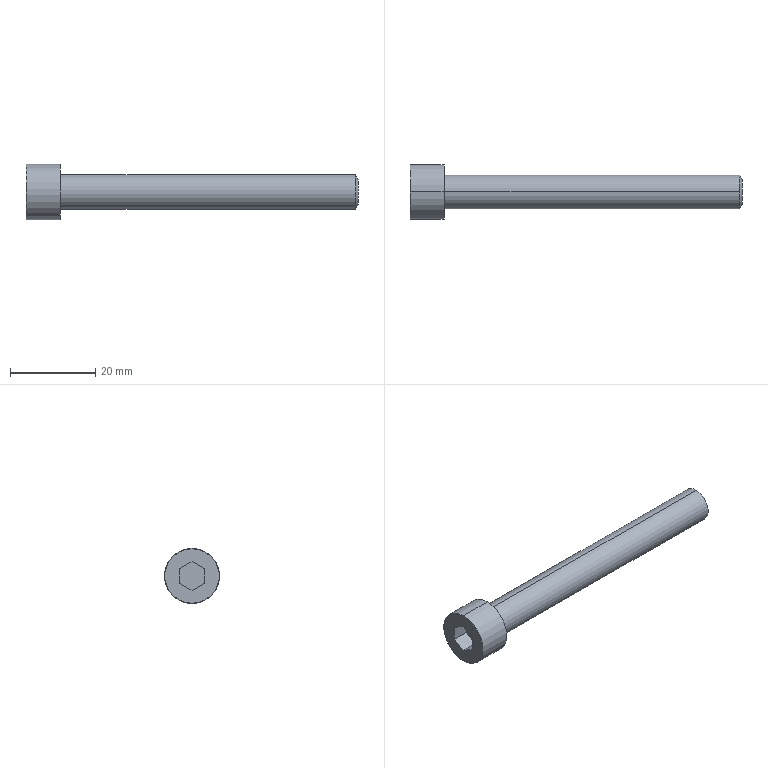Part | STEP file | 1 solid | 20 faces | box 78 x 13 x 13 mm | volume 4451 mm3 | plane 10 | torus 4 | cylinder 4 | cone 2 | commonest cylinder face diameters 8 x2 13 x2
STEP:
#1=CARTESIAN_POINT('',(0.,0.,6.4));
#2=VERTEX_POINT('',#1);
#3=CARTESIAN_POINT('',(0.,0.,-6.4));
#4=VERTEX_POINT('',#3);
#5=CARTESIAN_POINT('',(0.,0.,0.));
#6=DIRECTION('',(-1.,0.,0.));
#7=DIRECTION('',(0.,0.,-1.));
#8=AXIS2_PLACEMENT_3D('',#5,#6,#7);
#9=CIRCLE('',#8,6.4);
#10=EDGE_CURVE('',#2,#4,#9,.T.);
#11=ORIENTED_EDGE('',*,*,#10,.F.);
#12=CARTESIAN_POINT('',(0.1,0.,6.5));
#13=VERTEX_POINT('',#12);
#14=CARTESIAN_POINT('',(0.1,0.,6.4));
#15=DIRECTION('',(0.,1.,0.));
#16=DIRECTION('',(0.,0.,1.));
#17=AXIS2_PLACEMENT_3D('',#14,#15,#16);
#18=CIRCLE('',#17,0.1);
#19=EDGE_CURVE('',#2,#13,#18,.T.);
#20=ORIENTED_EDGE('',*,*,#19,.T.);
#21=CARTESIAN_POINT('',(0.1,0.,-6.5));
#22=VERTEX_POINT('',#21);
#23=CARTESIAN_POINT('',(0.1,0.,0.));
#24=DIRECTION('',(1.,0.,0.));
#25=DIRECTION('',(0.,0.,-1.));
#26=AXIS2_PLACEMENT_3D('',#23,#24,#25);
#27=CIRCLE('',#26,6.5);
#28=EDGE_CURVE('',#22,#13,#27,.T.);
#29=ORIENTED_EDGE('',*,*,#28,.F.);
#30=CARTESIAN_POINT('',(0.1,0.,-6.4));
#31=DIRECTION('',(0.,-1.,0.));
#32=DIRECTION('',(0.,0.,-1.));
#33=AXIS2_PLACEMENT_3D('',#30,#31,#32);
#34=CIRCLE('',#33,0.1);
#35=EDGE_CURVE('',#4,#22,#34,.T.);
#36=ORIENTED_EDGE('',*,*,#35,.F.);
#37=EDGE_LOOP('',(#11,#20,#29,#36));
#38=FACE_OUTER_BOUND('',#37,.T.);
#39=CARTESIAN_POINT('',(0.1,0.,0.));
#40=DIRECTION('',(1.,0.,0.));
#41=DIRECTION('',(0.,0.,-1.));
#42=AXIS2_PLACEMENT_3D('',#39,#40,#41);
#43=TOROIDAL_SURFACE('',#42,6.4,0.1);
#44=ADVANCED_FACE('',(#38),#43,.T.);
#45=CARTESIAN_POINT('',(78.,0.,2.917));
#46=VERTEX_POINT('',#45);
#47=CARTESIAN_POINT('',(78.,0.,-2.917));
#48=VERTEX_POINT('',#47);
#49=CARTESIAN_POINT('',(78.,0.,0.));
#50=DIRECTION('',(-1.,0.,0.));
#51=DIRECTION('',(0.,0.,1.));
#52=AXIS2_PLACEMENT_3D('',#49,#50,#51);
#53=CIRCLE('',#52,2.917);
#54=EDGE_CURVE('',#46,#48,#53,.T.);
#55=ORIENTED_EDGE('',*,*,#54,.T.);
#56=CARTESIAN_POINT('',(77.375,0.,-4.));
#57=VERTEX_POINT('',#56);
#58=CARTESIAN_POINT('',(77.375,0.,-4.));
#59=DIRECTION('',(-0.5,0.,-0.866));
#60=VECTOR('',#59,1000.);
#61=LINE('',#58,#60);
#62=EDGE_CURVE('',#48,#57,#61,.T.);
#63=ORIENTED_EDGE('',*,*,#62,.T.);
#64=CARTESIAN_POINT('',(77.375,0.,4.));
#65=VERTEX_POINT('',#64);
#66=CARTESIAN_POINT('',(77.375,0.,0.));
#67=DIRECTION('',(-1.,0.,0.));
#68=DIRECTION('',(0.,0.,1.));
#69=AXIS2_PLACEMENT_3D('',#66,#67,#68);
#70=CIRCLE('',#69,4.);
#71=EDGE_CURVE('',#65,#57,#70,.T.);
#72=ORIENTED_EDGE('',*,*,#71,.F.);
#73=CARTESIAN_POINT('',(77.375,0.,4.));
#74=DIRECTION('',(-0.5,0.,0.866));
#75=VECTOR('',#74,1000.);
#76=LINE('',#73,#75);
#77=EDGE_CURVE('',#46,#65,#76,.T.);
#78=ORIENTED_EDGE('',*,*,#77,.F.);
#79=EDGE_LOOP('',(#55,#63,#72,#78));
#80=FACE_OUTER_BOUND('',#79,.T.);
#81=CARTESIAN_POINT('',(77.375,0.,0.));
#82=DIRECTION('',(-1.,0.,0.));
#83=DIRECTION('',(0.,0.,1.));
#84=AXIS2_PLACEMENT_3D('',#81,#82,#83);
#85=CONICAL_SURFACE('',#84,4.,1.047);
#86=ADVANCED_FACE('',(#80),#85,.T.);
#87=CARTESIAN_POINT('',(8.,0.,-4.2));
#88=VERTEX_POINT('',#87);
#89=CARTESIAN_POINT('',(8.,0.,4.2));
#90=VERTEX_POINT('',#89);
#91=CARTESIAN_POINT('',(8.,0.,0.));
#92=DIRECTION('',(-1.,0.,0.));
#93=DIRECTION('',(0.,0.,1.));
#94=AXIS2_PLACEMENT_3D('',#91,#92,#93);
#95=CIRCLE('',#94,4.2);
#96=EDGE_CURVE('',#88,#90,#95,.T.);
#97=ORIENTED_EDGE('',*,*,#96,.F.);
#98=CARTESIAN_POINT('',(8.2,0.,-4.));
#99=VERTEX_POINT('',#98);
#100=CARTESIAN_POINT('',(8.2,0.,-4.2));
#101=DIRECTION('',(0.,1.,0.));
#102=DIRECTION('',(0.,0.,1.));
#103=AXIS2_PLACEMENT_3D('',#100,#101,#102);
#104=CIRCLE('',#103,0.2);
#105=EDGE_CURVE('',#88,#99,#104,.T.);
#106=ORIENTED_EDGE('',*,*,#105,.T.);
#107=CARTESIAN_POINT('',(8.2,0.,4.));
#108=VERTEX_POINT('',#107);
#109=CARTESIAN_POINT('',(8.2,0.,0.));
#110=DIRECTION('',(-1.,0.,0.));
#111=DIRECTION('',(0.,0.,1.));
#112=AXIS2_PLACEMENT_3D('',#109,#110,#111);
#113=CIRCLE('',#112,4.);
#114=EDGE_CURVE('',#99,#108,#113,.T.);
#115=ORIENTED_EDGE('',*,*,#114,.T.);
#116=CARTESIAN_POINT('',(8.2,0.,4.2));
#117=DIRECTION('',(0.,-1.,0.));
#118=DIRECTION('',(0.,0.,-1.));
#119=AXIS2_PLACEMENT_3D('',#116,#117,#118);
#120=CIRCLE('',#119,0.2);
#121=EDGE_CURVE('',#90,#108,#120,.T.);
#122=ORIENTED_EDGE('',*,*,#121,.F.);
#123=EDGE_LOOP('',(#97,#106,#115,#122));
#124=FACE_OUTER_BOUND('',#123,.T.);
#125=CARTESIAN_POINT('',(8.2,0.,0.));
#126=DIRECTION('',(-1.,0.,0.));
#127=DIRECTION('',(0.,0.,1.));
#128=AXIS2_PLACEMENT_3D('',#125,#126,#127);
#129=TOROIDAL_SURFACE('',#128,4.2,0.2);
#130=ADVANCED_FACE('',(#124),#129,.F.);
#131=CARTESIAN_POINT('',(8.,0.,6.5));
#132=VERTEX_POINT('',#131);
#133=CARTESIAN_POINT('',(8.,0.,-6.5));
#134=VERTEX_POINT('',#133);
#135=CARTESIAN_POINT('',(8.,0.,0.));
#136=DIRECTION('',(-1.,0.,0.));
#137=DIRECTION('',(0.,0.,1.));
#138=AXIS2_PLACEMENT_3D('',#135,#136,#137);
#139=CIRCLE('',#138,6.5);
#140=EDGE_CURVE('',#132,#134,#139,.T.);
#141=ORIENTED_EDGE('',*,*,#140,.T.);
#142=CARTESIAN_POINT('',(0.,0.,-6.5));
#143=DIRECTION('',(-1.,0.,0.));
#144=VECTOR('',#143,1000.);
#145=LINE('',#142,#144);
#146=EDGE_CURVE('',#134,#22,#145,.T.);
#147=ORIENTED_EDGE('',*,*,#146,.T.);
#148=ORIENTED_EDGE('',*,*,#28,.T.);
#149=CARTESIAN_POINT('',(0.,0.,6.5));
#150=DIRECTION('',(-1.,0.,0.));
#151=VECTOR('',#150,1000.);
#152=LINE('',#149,#151);
#153=EDGE_CURVE('',#132,#13,#152,.T.);
#154=ORIENTED_EDGE('',*,*,#153,.F.);
#155=EDGE_LOOP('',(#141,#147,#148,#154));
#156=FACE_OUTER_BOUND('',#155,.T.);
#157=CARTESIAN_POINT('',(0.,0.,0.));
#158=DIRECTION('',(-1.,0.,0.));
#159=DIRECTION('',(0.,0.,1.));
#160=AXIS2_PLACEMENT_3D('',#157,#158,#159);
#161=CYLINDRICAL_SURFACE('',#160,6.5);
#162=ADVANCED_FACE('',(#156),#161,.T.);
#163=ORIENTED_EDGE('',*,*,#71,.T.);
#164=CARTESIAN_POINT('',(0.,0.,-4.));
#165=DIRECTION('',(-1.,0.,0.));
#166=VECTOR('',#165,1000.);
#167=LINE('',#164,#166);
#168=EDGE_CURVE('',#57,#99,#167,.T.);
#169=ORIENTED_EDGE('',*,*,#168,.T.);
#170=CARTESIAN_POINT('',(8.2,0.,0.));
#171=DIRECTION('',(-1.,0.,0.));
#172=DIRECTION('',(0.,0.,1.));
#173=AXIS2_PLACEMENT_3D('',#170,#171,#172);
#174=CIRCLE('',#173,4.);
#175=EDGE_CURVE('',#108,#99,#174,.T.);
#176=ORIENTED_EDGE('',*,*,#175,.F.);
#177=CARTESIAN_POINT('',(0.,0.,4.));
#178=DIRECTION('',(-1.,0.,0.));
#179=VECTOR('',#178,1000.);
#180=LINE('',#177,#179);
#181=EDGE_CURVE('',#65,#108,#180,.T.);
#182=ORIENTED_EDGE('',*,*,#181,.F.);
#183=EDGE_LOOP('',(#163,#169,#176,#182));
#184=FACE_OUTER_BOUND('',#183,.T.);
#185=CARTESIAN_POINT('',(0.,0.,0.));
#186=DIRECTION('',(-1.,0.,0.));
#187=DIRECTION('',(0.,0.,1.));
#188=AXIS2_PLACEMENT_3D('',#185,#186,#187);
#189=CYLINDRICAL_SURFACE('',#188,4.);
#190=ADVANCED_FACE('',(#184),#189,.T.);
#191=ORIENTED_EDGE('',*,*,#168,.F.);
#192=CARTESIAN_POINT('',(77.375,0.,0.));
#193=DIRECTION('',(-1.,0.,0.));
#194=DIRECTION('',(0.,0.,1.));
#195=AXIS2_PLACEMENT_3D('',#192,#193,#194);
#196=CIRCLE('',#195,4.);
#197=EDGE_CURVE('',#57,#65,#196,.T.);
#198=ORIENTED_EDGE('',*,*,#197,.T.);
#199=ORIENTED_EDGE('',*,*,#181,.T.);
#200=ORIENTED_EDGE('',*,*,#114,.F.);
#201=EDGE_LOOP('',(#191,#198,#199,#200));
#202=FACE_OUTER_BOUND('',#201,.T.);
#203=CARTESIAN_POINT('',(0.,0.,0.));
#204=DIRECTION('',(-1.,0.,0.));
#205=DIRECTION('',(0.,0.,1.));
#206=AXIS2_PLACEMENT_3D('',#203,#204,#205);
#207=CYLINDRICAL_SURFACE('',#206,4.);
#208=ADVANCED_FACE('',(#202),#207,.T.);
#209=CARTESIAN_POINT('',(0.,0.,0.));
#210=DIRECTION('',(-1.,0.,0.));
#211=DIRECTION('',(0.,0.,-1.));
#212=AXIS2_PLACEMENT_3D('',#209,#210,#211);
#213=CIRCLE('',#212,6.4);
#214=EDGE_CURVE('',#4,#2,#213,.T.);
#215=ORIENTED_EDGE('',*,*,#214,.T.);
#216=ORIENTED_EDGE('',*,*,#10,.T.);
#217=EDGE_LOOP('',(#215,#216));
#218=FACE_OUTER_BOUND('',#217,.T.);
#219=CARTESIAN_POINT('',(0.,0.,3.43));
#220=VERTEX_POINT('',#219);
#221=CARTESIAN_POINT('',(0.,2.97,1.715));
#222=VERTEX_POINT('',#221);
#223=CARTESIAN_POINT('',(0.,0.,3.43));
#224=DIRECTION('',(0.,0.866,-0.5));
#225=VECTOR('',#224,1000.);
#226=LINE('',#223,#225);
#227=EDGE_CURVE('',#220,#222,#226,.T.);
#228=ORIENTED_EDGE('',*,*,#227,.F.);
#229=CARTESIAN_POINT('',(0.,-2.97,1.715));
#230=VERTEX_POINT('',#229);
#231=CARTESIAN_POINT('',(0.,-2.97,1.715));
#232=DIRECTION('',(0.,0.866,0.5));
#233=VECTOR('',#232,1000.);
#234=LINE('',#231,#233);
#235=EDGE_CURVE('',#230,#220,#234,.T.);
#236=ORIENTED_EDGE('',*,*,#235,.F.);
#237=CARTESIAN_POINT('',(0.,-2.97,-1.715));
#238=VERTEX_POINT('',#237);
#239=CARTESIAN_POINT('',(0.,-2.97,-1.715));
#240=DIRECTION('',(0.,0.,1.));
#241=VECTOR('',#240,1000.);
#242=LINE('',#239,#241);
#243=EDGE_CURVE('',#238,#230,#242,.T.);
#244=ORIENTED_EDGE('',*,*,#243,.F.);
#245=CARTESIAN_POINT('',(0.,0.,-3.43));
#246=VERTEX_POINT('',#245);
#247=CARTESIAN_POINT('',(0.,0.,-3.43));
#248=DIRECTION('',(0.,-0.866,0.5));
#249=VECTOR('',#248,1000.);
#250=LINE('',#247,#249);
#251=EDGE_CURVE('',#246,#238,#250,.T.);
#252=ORIENTED_EDGE('',*,*,#251,.F.);
#253=CARTESIAN_POINT('',(0.,2.97,-1.715));
#254=VERTEX_POINT('',#253);
#255=CARTESIAN_POINT('',(0.,2.97,-1.715));
#256=DIRECTION('',(0.,-0.866,-0.5));
#257=VECTOR('',#256,1000.);
#258=LINE('',#255,#257);
#259=EDGE_CURVE('',#254,#246,#258,.T.);
#260=ORIENTED_EDGE('',*,*,#259,.F.);
#261=CARTESIAN_POINT('',(0.,2.97,1.715));
#262=DIRECTION('',(0.,0.,-1.));
#263=VECTOR('',#262,1000.);
#264=LINE('',#261,#263);
#265=EDGE_CURVE('',#222,#254,#264,.T.);
#266=ORIENTED_EDGE('',*,*,#265,.F.);
#267=EDGE_LOOP('',(#228,#236,#244,#252,#260,#266));
#268=FACE_BOUND('',#267,.T.);
#269=CARTESIAN_POINT('',(0.,0.,0.));
#270=DIRECTION('',(1.,0.,0.));
#271=DIRECTION('',(0.,0.,-1.));
#272=AXIS2_PLACEMENT_3D('',#269,#270,#271);
#273=PLANE('',#272);
#274=ADVANCED_FACE('',(#218,#268),#273,.F.);
#275=ORIENTED_EDGE('',*,*,#146,.F.);
#276=CARTESIAN_POINT('',(8.,0.,0.));
#277=DIRECTION('',(-1.,0.,0.));
#278=DIRECTION('',(0.,0.,1.));
#279=AXIS2_PLACEMENT_3D('',#276,#277,#278);
#280=CIRCLE('',#279,6.5);
#281=EDGE_CURVE('',#134,#132,#280,.T.);
#282=ORIENTED_EDGE('',*,*,#281,.T.);
#283=ORIENTED_EDGE('',*,*,#153,.T.);
#284=CARTESIAN_POINT('',(0.1,0.,0.));
#285=DIRECTION('',(1.,0.,0.));
#286=DIRECTION('',(0.,0.,-1.));
#287=AXIS2_PLACEMENT_3D('',#284,#285,#286);
#288=CIRCLE('',#287,6.5);
#289=EDGE_CURVE('',#13,#22,#288,.T.);
#290=ORIENTED_EDGE('',*,*,#289,.T.);
#291=EDGE_LOOP('',(#275,#282,#283,#290));
#292=FACE_OUTER_BOUND('',#291,.T.);
#293=CARTESIAN_POINT('',(0.,0.,0.));
#294=DIRECTION('',(-1.,0.,0.));
#295=DIRECTION('',(0.,0.,1.));
#296=AXIS2_PLACEMENT_3D('',#293,#294,#295);
#297=CYLINDRICAL_SURFACE('',#296,6.5);
#298=ADVANCED_FACE('',(#292),#297,.T.);
#299=ORIENTED_EDGE('',*,*,#140,.F.);
#300=ORIENTED_EDGE('',*,*,#281,.F.);
#301=EDGE_LOOP('',(#299,#300));
#302=FACE_OUTER_BOUND('',#301,.T.);
#303=CARTESIAN_POINT('',(8.,0.,0.));
#304=DIRECTION('',(-1.,0.,0.));
#305=DIRECTION('',(0.,0.,1.));
#306=AXIS2_PLACEMENT_3D('',#303,#304,#305);
#307=CIRCLE('',#306,4.2);
#308=EDGE_CURVE('',#90,#88,#307,.T.);
#309=ORIENTED_EDGE('',*,*,#308,.T.);
#310=ORIENTED_EDGE('',*,*,#96,.T.);
#311=EDGE_LOOP('',(#309,#310));
#312=FACE_BOUND('',#311,.T.);
#313=CARTESIAN_POINT('',(8.,6.5,0.));
#314=DIRECTION('',(-1.,0.,0.));
#315=DIRECTION('',(0.,0.,1.));
#316=AXIS2_PLACEMENT_3D('',#313,#314,#315);
#317=PLANE('',#316);
#318=ADVANCED_FACE('',(#302,#312),#317,.F.);
#319=ORIENTED_EDGE('',*,*,#105,.F.);
#320=ORIENTED_EDGE('',*,*,#308,.F.);
#321=ORIENTED_EDGE('',*,*,#121,.T.);
#322=ORIENTED_EDGE('',*,*,#175,.T.);
#323=EDGE_LOOP('',(#319,#320,#321,#322));
#324=FACE_OUTER_BOUND('',#323,.T.);
#325=CARTESIAN_POINT('',(8.2,0.,0.));
#326=DIRECTION('',(-1.,0.,0.));
#327=DIRECTION('',(0.,0.,1.));
#328=AXIS2_PLACEMENT_3D('',#325,#326,#327);
#329=TOROIDAL_SURFACE('',#328,4.2,0.2);
#330=ADVANCED_FACE('',(#324),#329,.F.);
#331=ORIENTED_EDGE('',*,*,#235,.T.);
#332=CARTESIAN_POINT('',(4.,0.,3.43));
#333=VERTEX_POINT('',#332);
#334=CARTESIAN_POINT('',(4.,0.,3.43));
#335=DIRECTION('',(-1.,0.,0.));
#336=VECTOR('',#335,1000.);
#337=LINE('',#334,#336);
#338=EDGE_CURVE('',#333,#220,#337,.T.);
#339=ORIENTED_EDGE('',*,*,#338,.F.);
#340=CARTESIAN_POINT('',(4.,-2.97,1.715));
#341=VERTEX_POINT('',#340);
#342=CARTESIAN_POINT('',(4.,-2.97,1.715));
#343=DIRECTION('',(0.,0.866,0.5));
#344=VECTOR('',#343,1000.);
#345=LINE('',#342,#344);
#346=EDGE_CURVE('',#341,#333,#345,.T.);
#347=ORIENTED_EDGE('',*,*,#346,.F.);
#348=CARTESIAN_POINT('',(4.,-2.97,1.715));
#349=DIRECTION('',(-1.,0.,0.));
#350=VECTOR('',#349,1000.);
#351=LINE('',#348,#350);
#352=EDGE_CURVE('',#341,#230,#351,.T.);
#353=ORIENTED_EDGE('',*,*,#352,.T.);
#354=EDGE_LOOP('',(#331,#339,#347,#353));
#355=FACE_OUTER_BOUND('',#354,.T.);
#356=CARTESIAN_POINT('',(4.,-2.97,1.715));
#357=DIRECTION('',(0.,-0.5,0.866));
#358=DIRECTION('',(0.,-0.866,-0.5));
#359=AXIS2_PLACEMENT_3D('',#356,#357,#358);
#360=PLANE('',#359);
#361=ADVANCED_FACE('',(#355),#360,.F.);
#362=ORIENTED_EDGE('',*,*,#243,.T.);
#363=ORIENTED_EDGE('',*,*,#352,.F.);
#364=CARTESIAN_POINT('',(4.,-2.97,-1.715));
#365=VERTEX_POINT('',#364);
#366=CARTESIAN_POINT('',(4.,-2.97,-1.715));
#367=DIRECTION('',(0.,0.,1.));
#368=VECTOR('',#367,1000.);
#369=LINE('',#366,#368);
#370=EDGE_CURVE('',#365,#341,#369,.T.);
#371=ORIENTED_EDGE('',*,*,#370,.F.);
#372=CARTESIAN_POINT('',(4.,-2.97,-1.715));
#373=DIRECTION('',(-1.,0.,0.));
#374=VECTOR('',#373,1000.);
#375=LINE('',#372,#374);
#376=EDGE_CURVE('',#365,#238,#375,.T.);
#377=ORIENTED_EDGE('',*,*,#376,.T.);
#378=EDGE_LOOP('',(#362,#363,#371,#377));
#379=FACE_OUTER_BOUND('',#378,.T.);
#380=CARTESIAN_POINT('',(4.,-2.97,-1.715));
#381=DIRECTION('',(0.,-1.,0.));
#382=DIRECTION('',(0.,0.,-1.));
#383=AXIS2_PLACEMENT_3D('',#380,#381,#382);
#384=PLANE('',#383);
#385=ADVANCED_FACE('',(#379),#384,.F.);
#386=ORIENTED_EDGE('',*,*,#251,.T.);
#387=ORIENTED_EDGE('',*,*,#376,.F.);
#388=CARTESIAN_POINT('',(4.,0.,-3.43));
#389=VERTEX_POINT('',#388);
#390=CARTESIAN_POINT('',(4.,0.,-3.43));
#391=DIRECTION('',(0.,-0.866,0.5));
#392=VECTOR('',#391,1000.);
#393=LINE('',#390,#392);
#394=EDGE_CURVE('',#389,#365,#393,.T.);
#395=ORIENTED_EDGE('',*,*,#394,.F.);
#396=CARTESIAN_POINT('',(4.,0.,-3.43));
#397=DIRECTION('',(-1.,0.,0.));
#398=VECTOR('',#397,1000.);
#399=LINE('',#396,#398);
#400=EDGE_CURVE('',#389,#246,#399,.T.);
#401=ORIENTED_EDGE('',*,*,#400,.T.);
#402=EDGE_LOOP('',(#386,#387,#395,#401));
#403=FACE_OUTER_BOUND('',#402,.T.);
#404=CARTESIAN_POINT('',(4.,0.,-3.43));
#405=DIRECTION('',(0.,-0.5,-0.866));
#406=DIRECTION('',(0.,0.866,-0.5));
#407=AXIS2_PLACEMENT_3D('',#404,#405,#406);
#408=PLANE('',#407);
#409=ADVANCED_FACE('',(#403),#408,.F.);
#410=ORIENTED_EDGE('',*,*,#259,.T.);
#411=ORIENTED_EDGE('',*,*,#400,.F.);
#412=CARTESIAN_POINT('',(4.,2.97,-1.715));
#413=VERTEX_POINT('',#412);
#414=CARTESIAN_POINT('',(4.,2.97,-1.715));
#415=DIRECTION('',(0.,-0.866,-0.5));
#416=VECTOR('',#415,1000.);
#417=LINE('',#414,#416);
#418=EDGE_CURVE('',#413,#389,#417,.T.);
#419=ORIENTED_EDGE('',*,*,#418,.F.);
#420=CARTESIAN_POINT('',(4.,2.97,-1.715));
#421=DIRECTION('',(-1.,0.,0.));
#422=VECTOR('',#421,1000.);
#423=LINE('',#420,#422);
#424=EDGE_CURVE('',#413,#254,#423,.T.);
#425=ORIENTED_EDGE('',*,*,#424,.T.);
#426=EDGE_LOOP('',(#410,#411,#419,#425));
#427=FACE_OUTER_BOUND('',#426,.T.);
#428=CARTESIAN_POINT('',(4.,2.97,-1.715));
#429=DIRECTION('',(0.,0.5,-0.866));
#430=DIRECTION('',(0.,0.866,0.5));
#431=AXIS2_PLACEMENT_3D('',#428,#429,#430);
#432=PLANE('',#431);
#433=ADVANCED_FACE('',(#427),#432,.F.);
#434=ORIENTED_EDGE('',*,*,#265,.T.);
#435=ORIENTED_EDGE('',*,*,#424,.F.);
#436=CARTESIAN_POINT('',(4.,2.97,1.715));
#437=VERTEX_POINT('',#436);
#438=CARTESIAN_POINT('',(4.,2.97,1.715));
#439=DIRECTION('',(0.,0.,-1.));
#440=VECTOR('',#439,1000.);
#441=LINE('',#438,#440);
#442=EDGE_CURVE('',#437,#413,#441,.T.);
#443=ORIENTED_EDGE('',*,*,#442,.F.);
#444=CARTESIAN_POINT('',(4.,2.97,1.715));
#445=DIRECTION('',(-1.,0.,0.));
#446=VECTOR('',#445,1000.);
#447=LINE('',#444,#446);
#448=EDGE_CURVE('',#437,#222,#447,.T.);
#449=ORIENTED_EDGE('',*,*,#448,.T.);
#450=EDGE_LOOP('',(#434,#435,#443,#449));
#451=FACE_OUTER_BOUND('',#450,.T.);
#452=CARTESIAN_POINT('',(4.,2.97,1.715));
#453=DIRECTION('',(0.,1.,0.));
#454=DIRECTION('',(0.,0.,1.));
#455=AXIS2_PLACEMENT_3D('',#452,#453,#454);
#456=PLANE('',#455);
#457=ADVANCED_FACE('',(#451),#456,.F.);
#458=ORIENTED_EDGE('',*,*,#227,.T.);
#459=ORIENTED_EDGE('',*,*,#448,.F.);
#460=CARTESIAN_POINT('',(4.,0.,3.43));
#461=DIRECTION('',(0.,0.866,-0.5));
#462=VECTOR('',#461,1000.);
#463=LINE('',#460,#462);
#464=EDGE_CURVE('',#333,#437,#463,.T.);
#465=ORIENTED_EDGE('',*,*,#464,.F.);
#466=ORIENTED_EDGE('',*,*,#338,.T.);
#467=EDGE_LOOP('',(#458,#459,#465,#466));
#468=FACE_OUTER_BOUND('',#467,.T.);
#469=CARTESIAN_POINT('',(4.,0.,3.43));
#470=DIRECTION('',(0.,0.5,0.866));
#471=DIRECTION('',(0.,-0.866,0.5));
#472=AXIS2_PLACEMENT_3D('',#469,#470,#471);
#473=PLANE('',#472);
#474=ADVANCED_FACE('',(#468),#473,.F.);
#475=ORIENTED_EDGE('',*,*,#346,.T.);
#476=ORIENTED_EDGE('',*,*,#464,.T.);
#477=ORIENTED_EDGE('',*,*,#442,.T.);
#478=ORIENTED_EDGE('',*,*,#418,.T.);
#479=ORIENTED_EDGE('',*,*,#394,.T.);
#480=ORIENTED_EDGE('',*,*,#370,.T.);
#481=EDGE_LOOP('',(#475,#476,#477,#478,#479,#480));
#482=FACE_OUTER_BOUND('',#481,.T.);
#483=CARTESIAN_POINT('',(4.,-2.97,1.715));
#484=DIRECTION('',(1.,0.,0.));
#485=DIRECTION('',(0.,0.,-1.));
#486=AXIS2_PLACEMENT_3D('',#483,#484,#485);
#487=PLANE('',#486);
#488=ADVANCED_FACE('',(#482),#487,.F.);
#489=ORIENTED_EDGE('',*,*,#62,.F.);
#490=CARTESIAN_POINT('',(78.,0.,0.));
#491=DIRECTION('',(-1.,0.,0.));
#492=DIRECTION('',(0.,0.,1.));
#493=AXIS2_PLACEMENT_3D('',#490,#491,#492);
#494=CIRCLE('',#493,2.917);
#495=EDGE_CURVE('',#48,#46,#494,.T.);
#496=ORIENTED_EDGE('',*,*,#495,.T.);
#497=ORIENTED_EDGE('',*,*,#77,.T.);
#498=ORIENTED_EDGE('',*,*,#197,.F.);
#499=EDGE_LOOP('',(#489,#496,#497,#498));
#500=FACE_OUTER_BOUND('',#499,.T.);
#501=CARTESIAN_POINT('',(77.375,0.,0.));
#502=DIRECTION('',(-1.,0.,0.));
#503=DIRECTION('',(0.,0.,1.));
#504=AXIS2_PLACEMENT_3D('',#501,#502,#503);
#505=CONICAL_SURFACE('',#504,4.,1.047);
#506=ADVANCED_FACE('',(#500),#505,.T.);
#507=ORIENTED_EDGE('',*,*,#54,.F.);
#508=ORIENTED_EDGE('',*,*,#495,.F.);
#509=EDGE_LOOP('',(#507,#508));
#510=FACE_OUTER_BOUND('',#509,.T.);
#511=CARTESIAN_POINT('',(78.,4.,0.));
#512=DIRECTION('',(-1.,0.,0.));
#513=DIRECTION('',(0.,0.,1.));
#514=AXIS2_PLACEMENT_3D('',#511,#512,#513);
#515=PLANE('',#514);
#516=ADVANCED_FACE('',(#510),#515,.F.);
#517=ORIENTED_EDGE('',*,*,#19,.F.);
#518=ORIENTED_EDGE('',*,*,#214,.F.);
#519=ORIENTED_EDGE('',*,*,#35,.T.);
#520=ORIENTED_EDGE('',*,*,#289,.F.);
#521=EDGE_LOOP('',(#517,#518,#519,#520));
#522=FACE_OUTER_BOUND('',#521,.T.);
#523=CARTESIAN_POINT('',(0.1,0.,0.));
#524=DIRECTION('',(1.,0.,0.));
#525=DIRECTION('',(0.,0.,-1.));
#526=AXIS2_PLACEMENT_3D('',#523,#524,#525);
#527=TOROIDAL_SURFACE('',#526,6.4,0.1);
#528=ADVANCED_FACE('',(#522),#527,.T.);
#529=CLOSED_SHELL('',(#44,#86,#130,#162,#190,#208,#274,#298,#318,#330,#361,#385,#409,#433,#457,#474,#488,#506,#516,#528));
#530=MANIFOLD_SOLID_BREP('',#529);
#531=CARTESIAN_POINT('',(0.,0.,0.));
#532=DIRECTION('',(0.,0.,1.));
#533=DIRECTION('',(1.,0.,0.));
#534=AXIS2_PLACEMENT_3D('',#531,#532,#533);
#535=(LENGTH_UNIT()NAMED_UNIT(*)SI_UNIT(.MILLI.,.METRE.));
#536=UNCERTAINTY_MEASURE_WITH_UNIT(LENGTH_MEASURE(0.00001),#535,'','');
#537=(NAMED_UNIT(*)PLANE_ANGLE_UNIT()SI_UNIT($,.RADIAN.));
#538=(NAMED_UNIT(*)SI_UNIT($,.STERADIAN.)SOLID_ANGLE_UNIT());
#539=(GEOMETRIC_REPRESENTATION_CONTEXT(3)GLOBAL_UNCERTAINTY_ASSIGNED_CONTEXT((#536))GLOBAL_UNIT_ASSIGNED_CONTEXT((#535,#537,#538))REPRESENTATION_CONTEXT('',''));
#540=ADVANCED_BREP_SHAPE_REPRESENTATION('',(#530,#534),#539);